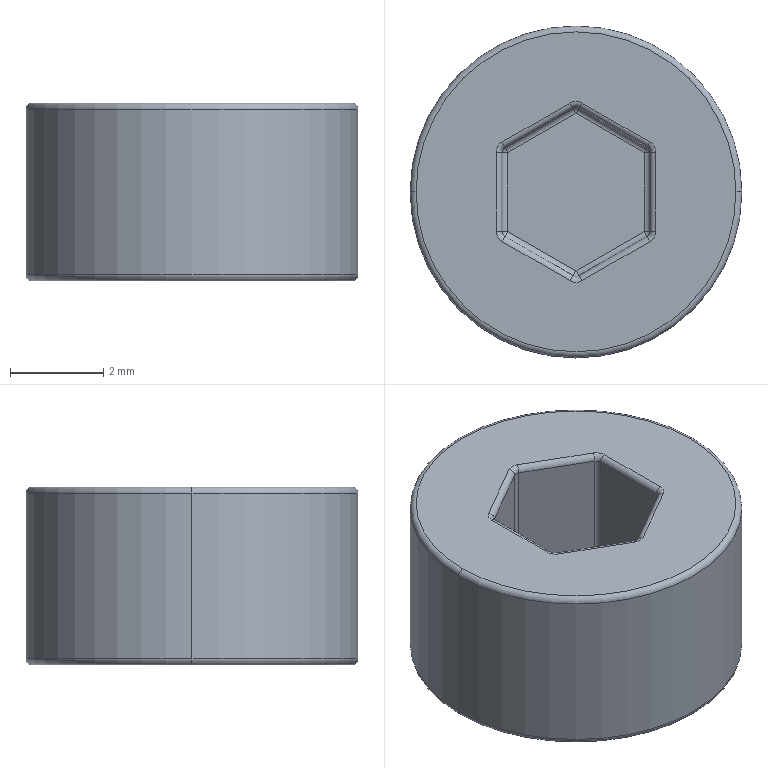Part | STEP file | BOLT | 1 solid | 45 faces | box 7.112 x 7.112 x 3.81 mm | volume 129.04 mm3 | cylinder 20 | torus 10 | plane 9 | sphere 6 | commonest cylinder face diameters 0.254 x18 7.112 x2
STEP:
#1=CARTESIAN_POINT('',(-3.556,0.,-0.127));
#2=VERTEX_POINT('',#1);
#3=CARTESIAN_POINT('',(3.556,0.,-0.127));
#4=VERTEX_POINT('',#3);
#5=CARTESIAN_POINT('',(0.,0.,-0.127));
#6=DIRECTION('',(0.,0.,-1.));
#7=DIRECTION('',(1.,0.,0.));
#8=AXIS2_PLACEMENT_3D('',#5,#6,#7);
#9=CIRCLE('',#8,3.556);
#10=EDGE_CURVE('',#2,#4,#9,.T.);
#11=ORIENTED_EDGE('',*,*,#10,.F.);
#12=CARTESIAN_POINT('',(-3.429,0.,0.));
#13=VERTEX_POINT('',#12);
#14=CARTESIAN_POINT('',(-3.429,0.,-0.127));
#15=DIRECTION('',(0.,1.,0.));
#16=DIRECTION('',(-1.,0.,0.));
#17=AXIS2_PLACEMENT_3D('',#14,#15,#16);
#18=CIRCLE('',#17,0.127);
#19=EDGE_CURVE('',#2,#13,#18,.T.);
#20=ORIENTED_EDGE('',*,*,#19,.T.);
#21=CARTESIAN_POINT('',(3.429,0.,0.));
#22=VERTEX_POINT('',#21);
#23=CARTESIAN_POINT('',(0.,0.,0.));
#24=DIRECTION('',(0.,0.,1.));
#25=DIRECTION('',(1.,0.,0.));
#26=AXIS2_PLACEMENT_3D('',#23,#24,#25);
#27=CIRCLE('',#26,3.429);
#28=EDGE_CURVE('',#22,#13,#27,.T.);
#29=ORIENTED_EDGE('',*,*,#28,.F.);
#30=CARTESIAN_POINT('',(3.429,0.,-0.127));
#31=DIRECTION('',(0.,-1.,0.));
#32=DIRECTION('',(0.,0.,-1.));
#33=AXIS2_PLACEMENT_3D('',#30,#31,#32);
#34=CIRCLE('',#33,0.127);
#35=EDGE_CURVE('',#4,#22,#34,.T.);
#36=ORIENTED_EDGE('',*,*,#35,.F.);
#37=EDGE_LOOP('',(#11,#20,#29,#36));
#38=FACE_OUTER_BOUND('',#37,.T.);
#39=CARTESIAN_POINT('',(0.,0.,-0.127));
#40=DIRECTION('',(0.,0.,1.));
#41=DIRECTION('',(1.,0.,0.));
#42=AXIS2_PLACEMENT_3D('',#39,#40,#41);
#43=TOROIDAL_SURFACE('',#42,3.429,0.127);
#44=ADVANCED_FACE('',(#38),#43,.T.);
#45=CARTESIAN_POINT('',(-3.429,0.,-3.81));
#46=VERTEX_POINT('',#45);
#47=CARTESIAN_POINT('',(3.429,0.,-3.81));
#48=VERTEX_POINT('',#47);
#49=CARTESIAN_POINT('',(0.,0.,-3.81));
#50=DIRECTION('',(0.,0.,-1.));
#51=DIRECTION('',(1.,0.,0.));
#52=AXIS2_PLACEMENT_3D('',#49,#50,#51);
#53=CIRCLE('',#52,3.429);
#54=EDGE_CURVE('',#46,#48,#53,.T.);
#55=ORIENTED_EDGE('',*,*,#54,.F.);
#56=CARTESIAN_POINT('',(-3.556,0.,-3.683));
#57=VERTEX_POINT('',#56);
#58=CARTESIAN_POINT('',(-3.429,0.,-3.683));
#59=DIRECTION('',(0.,1.,0.));
#60=DIRECTION('',(-1.,0.,0.));
#61=AXIS2_PLACEMENT_3D('',#58,#59,#60);
#62=CIRCLE('',#61,0.127);
#63=EDGE_CURVE('',#46,#57,#62,.T.);
#64=ORIENTED_EDGE('',*,*,#63,.T.);
#65=CARTESIAN_POINT('',(3.556,0.,-3.683));
#66=VERTEX_POINT('',#65);
#67=CARTESIAN_POINT('',(0.,0.,-3.683));
#68=DIRECTION('',(0.,0.,1.));
#69=DIRECTION('',(1.,0.,0.));
#70=AXIS2_PLACEMENT_3D('',#67,#68,#69);
#71=CIRCLE('',#70,3.556);
#72=EDGE_CURVE('',#66,#57,#71,.T.);
#73=ORIENTED_EDGE('',*,*,#72,.F.);
#74=CARTESIAN_POINT('',(3.429,0.,-3.683));
#75=DIRECTION('',(0.,-1.,0.));
#76=DIRECTION('',(0.,0.,-1.));
#77=AXIS2_PLACEMENT_3D('',#74,#75,#76);
#78=CIRCLE('',#77,0.127);
#79=EDGE_CURVE('',#48,#66,#78,.T.);
#80=ORIENTED_EDGE('',*,*,#79,.F.);
#81=EDGE_LOOP('',(#55,#64,#73,#80));
#82=FACE_OUTER_BOUND('',#81,.T.);
#83=CARTESIAN_POINT('',(0.,0.,-3.683));
#84=DIRECTION('',(0.,0.,1.));
#85=DIRECTION('',(1.,0.,0.));
#86=AXIS2_PLACEMENT_3D('',#83,#84,#85);
#87=TOROIDAL_SURFACE('',#86,3.429,0.127);
#88=ADVANCED_FACE('',(#82),#87,.T.);
#89=ORIENTED_EDGE('',*,*,#72,.T.);
#90=CARTESIAN_POINT('',(-3.556,0.,-3.81));
#91=DIRECTION('',(0.,0.,1.));
#92=VECTOR('',#91,1000.);
#93=LINE('',#90,#92);
#94=EDGE_CURVE('',#57,#2,#93,.T.);
#95=ORIENTED_EDGE('',*,*,#94,.T.);
#96=ORIENTED_EDGE('',*,*,#10,.T.);
#97=CARTESIAN_POINT('',(3.556,0.,-3.81));
#98=DIRECTION('',(0.,0.,1.));
#99=VECTOR('',#98,1000.);
#100=LINE('',#97,#99);
#101=EDGE_CURVE('',#66,#4,#100,.T.);
#102=ORIENTED_EDGE('',*,*,#101,.F.);
#103=EDGE_LOOP('',(#89,#95,#96,#102));
#104=FACE_OUTER_BOUND('',#103,.T.);
#105=CARTESIAN_POINT('',(0.,0.,-3.81));
#106=DIRECTION('',(0.,0.,1.));
#107=DIRECTION('',(1.,0.,0.));
#108=AXIS2_PLACEMENT_3D('',#105,#106,#107);
#109=CYLINDRICAL_SURFACE('',#108,3.556);
#110=ADVANCED_FACE('',(#104),#109,.T.);
#111=ORIENTED_EDGE('',*,*,#28,.T.);
#112=CARTESIAN_POINT('',(0.,0.,0.));
#113=DIRECTION('',(0.,0.,1.));
#114=DIRECTION('',(1.,0.,0.));
#115=AXIS2_PLACEMENT_3D('',#112,#113,#114);
#116=CIRCLE('',#115,3.429);
#117=EDGE_CURVE('',#13,#22,#116,.T.);
#118=ORIENTED_EDGE('',*,*,#117,.T.);
#119=EDGE_LOOP('',(#111,#118));
#120=FACE_OUTER_BOUND('',#119,.T.);
#121=CARTESIAN_POINT('',(1.587,-1.063,0.));
#122=VERTEX_POINT('',#121);
#123=CARTESIAN_POINT('',(1.715,-0.8432,0.));
#124=VERTEX_POINT('',#123);
#125=CARTESIAN_POINT('',(1.46,-0.8432,0.));
#126=DIRECTION('',(0.,0.,1.));
#127=DIRECTION('',(1.,0.,0.));
#128=AXIS2_PLACEMENT_3D('',#125,#126,#127);
#129=CIRCLE('',#128,0.254);
#130=EDGE_CURVE('',#122,#124,#129,.T.);
#131=ORIENTED_EDGE('',*,*,#130,.F.);
#132=CARTESIAN_POINT('',(0.127,-1.906,0.));
#133=VERTEX_POINT('',#132);
#134=CARTESIAN_POINT('',(0.8573,-1.485,0.));
#135=DIRECTION('',(-0.866,-0.5,0.));
#136=VECTOR('',#135,1000.);
#137=LINE('',#134,#136);
#138=EDGE_CURVE('',#122,#133,#137,.T.);
#139=ORIENTED_EDGE('',*,*,#138,.T.);
#140=CARTESIAN_POINT('',(-0.127,-1.906,0.));
#141=VERTEX_POINT('',#140);
#142=CARTESIAN_POINT('',(0.,-1.686,0.));
#143=DIRECTION('',(0.,0.,1.));
#144=DIRECTION('',(1.,0.,0.));
#145=AXIS2_PLACEMENT_3D('',#142,#143,#144);
#146=CIRCLE('',#145,0.254);
#147=EDGE_CURVE('',#141,#133,#146,.T.);
#148=ORIENTED_EDGE('',*,*,#147,.F.);
#149=CARTESIAN_POINT('',(-1.587,-1.063,0.));
#150=VERTEX_POINT('',#149);
#151=CARTESIAN_POINT('',(-0.8573,-1.485,0.));
#152=DIRECTION('',(-0.866,0.5,0.));
#153=VECTOR('',#152,1000.);
#154=LINE('',#151,#153);
#155=EDGE_CURVE('',#141,#150,#154,.T.);
#156=ORIENTED_EDGE('',*,*,#155,.T.);
#157=CARTESIAN_POINT('',(-1.715,-0.8432,0.));
#158=VERTEX_POINT('',#157);
#159=CARTESIAN_POINT('',(-1.46,-0.8432,0.));
#160=DIRECTION('',(0.,0.,1.));
#161=DIRECTION('',(1.,0.,0.));
#162=AXIS2_PLACEMENT_3D('',#159,#160,#161);
#163=CIRCLE('',#162,0.254);
#164=EDGE_CURVE('',#158,#150,#163,.T.);
#165=ORIENTED_EDGE('',*,*,#164,.F.);
#166=CARTESIAN_POINT('',(-1.715,0.8432,0.));
#167=VERTEX_POINT('',#166);
#168=CARTESIAN_POINT('',(-1.715,0.,0.));
#169=DIRECTION('',(0.,1.,0.));
#170=VECTOR('',#169,1000.);
#171=LINE('',#168,#170);
#172=EDGE_CURVE('',#158,#167,#171,.T.);
#173=ORIENTED_EDGE('',*,*,#172,.T.);
#174=CARTESIAN_POINT('',(-1.587,1.063,0.));
#175=VERTEX_POINT('',#174);
#176=CARTESIAN_POINT('',(-1.46,0.8432,0.));
#177=DIRECTION('',(0.,0.,1.));
#178=DIRECTION('',(1.,0.,0.));
#179=AXIS2_PLACEMENT_3D('',#176,#177,#178);
#180=CIRCLE('',#179,0.254);
#181=EDGE_CURVE('',#175,#167,#180,.T.);
#182=ORIENTED_EDGE('',*,*,#181,.F.);
#183=CARTESIAN_POINT('',(-0.127,1.906,0.));
#184=VERTEX_POINT('',#183);
#185=CARTESIAN_POINT('',(-0.8573,1.485,0.));
#186=DIRECTION('',(0.866,0.5,0.));
#187=VECTOR('',#186,1000.);
#188=LINE('',#185,#187);
#189=EDGE_CURVE('',#175,#184,#188,.T.);
#190=ORIENTED_EDGE('',*,*,#189,.T.);
#191=CARTESIAN_POINT('',(0.127,1.906,0.));
#192=VERTEX_POINT('',#191);
#193=CARTESIAN_POINT('',(0.,1.686,0.));
#194=DIRECTION('',(0.,0.,1.));
#195=DIRECTION('',(1.,0.,0.));
#196=AXIS2_PLACEMENT_3D('',#193,#194,#195);
#197=CIRCLE('',#196,0.254);
#198=EDGE_CURVE('',#192,#184,#197,.T.);
#199=ORIENTED_EDGE('',*,*,#198,.F.);
#200=CARTESIAN_POINT('',(1.587,1.063,0.));
#201=VERTEX_POINT('',#200);
#202=CARTESIAN_POINT('',(0.8573,1.485,0.));
#203=DIRECTION('',(0.866,-0.5,0.));
#204=VECTOR('',#203,1000.);
#205=LINE('',#202,#204);
#206=EDGE_CURVE('',#192,#201,#205,.T.);
#207=ORIENTED_EDGE('',*,*,#206,.T.);
#208=CARTESIAN_POINT('',(1.715,0.8432,0.));
#209=VERTEX_POINT('',#208);
#210=CARTESIAN_POINT('',(1.46,0.8432,0.));
#211=DIRECTION('',(0.,0.,1.));
#212=DIRECTION('',(1.,0.,0.));
#213=AXIS2_PLACEMENT_3D('',#210,#211,#212);
#214=CIRCLE('',#213,0.254);
#215=EDGE_CURVE('',#209,#201,#214,.T.);
#216=ORIENTED_EDGE('',*,*,#215,.F.);
#217=CARTESIAN_POINT('',(1.715,0.,0.));
#218=DIRECTION('',(0.,-1.,0.));
#219=VECTOR('',#218,1000.);
#220=LINE('',#217,#219);
#221=EDGE_CURVE('',#209,#124,#220,.T.);
#222=ORIENTED_EDGE('',*,*,#221,.T.);
#223=EDGE_LOOP('',(#131,#139,#148,#156,#165,#173,#182,#190,#199,#207,#216,#222));
#224=FACE_BOUND('',#223,.T.);
#225=CARTESIAN_POINT('',(0.,0.,0.));
#226=DIRECTION('',(0.,0.,1.));
#227=DIRECTION('',(1.,0.,0.));
#228=AXIS2_PLACEMENT_3D('',#225,#226,#227);
#229=PLANE('',#228);
#230=ADVANCED_FACE('',(#120,#224),#229,.T.);
#231=ORIENTED_EDGE('',*,*,#94,.F.);
#232=CARTESIAN_POINT('',(0.,0.,-3.683));
#233=DIRECTION('',(0.,0.,1.));
#234=DIRECTION('',(1.,0.,0.));
#235=AXIS2_PLACEMENT_3D('',#232,#233,#234);
#236=CIRCLE('',#235,3.556);
#237=EDGE_CURVE('',#57,#66,#236,.T.);
#238=ORIENTED_EDGE('',*,*,#237,.T.);
#239=ORIENTED_EDGE('',*,*,#101,.T.);
#240=CARTESIAN_POINT('',(0.,0.,-0.127));
#241=DIRECTION('',(0.,0.,-1.));
#242=DIRECTION('',(1.,0.,0.));
#243=AXIS2_PLACEMENT_3D('',#240,#241,#242);
#244=CIRCLE('',#243,3.556);
#245=EDGE_CURVE('',#4,#2,#244,.T.);
#246=ORIENTED_EDGE('',*,*,#245,.T.);
#247=EDGE_LOOP('',(#231,#238,#239,#246));
#248=FACE_OUTER_BOUND('',#247,.T.);
#249=CARTESIAN_POINT('',(0.,0.,-3.81));
#250=DIRECTION('',(0.,0.,1.));
#251=DIRECTION('',(1.,0.,0.));
#252=AXIS2_PLACEMENT_3D('',#249,#250,#251);
#253=CYLINDRICAL_SURFACE('',#252,3.556);
#254=ADVANCED_FACE('',(#248),#253,.T.);
#255=CARTESIAN_POINT('',(0.,0.,-3.81));
#256=DIRECTION('',(0.,0.,-1.));
#257=DIRECTION('',(1.,0.,0.));
#258=AXIS2_PLACEMENT_3D('',#255,#256,#257);
#259=CIRCLE('',#258,3.429);
#260=EDGE_CURVE('',#48,#46,#259,.T.);
#261=ORIENTED_EDGE('',*,*,#260,.T.);
#262=ORIENTED_EDGE('',*,*,#54,.T.);
#263=EDGE_LOOP('',(#261,#262));
#264=FACE_OUTER_BOUND('',#263,.T.);
#265=CARTESIAN_POINT('',(0.,0.,-3.81));
#266=DIRECTION('',(0.,0.,1.));
#267=DIRECTION('',(1.,0.,0.));
#268=AXIS2_PLACEMENT_3D('',#265,#266,#267);
#269=PLANE('',#268);
#270=ADVANCED_FACE('',(#264),#269,.F.);
#271=CARTESIAN_POINT('',(-1.587,0.8432,-0.127));
#272=VERTEX_POINT('',#271);
#273=CARTESIAN_POINT('',(-1.587,-0.8432,-0.127));
#274=VERTEX_POINT('',#273);
#275=CARTESIAN_POINT('',(-1.587,0.9165,-0.127));
#276=DIRECTION('',(0.,-1.,0.));
#277=VECTOR('',#276,1000.);
#278=LINE('',#275,#277);
#279=EDGE_CURVE('',#272,#274,#278,.T.);
#280=ORIENTED_EDGE('',*,*,#279,.T.);
#281=CARTESIAN_POINT('',(-1.587,-0.8432,-2.413));
#282=VERTEX_POINT('',#281);
#283=CARTESIAN_POINT('',(-1.587,-0.8432,-2.54));
#284=DIRECTION('',(0.,0.,-1.));
#285=VECTOR('',#284,1000.);
#286=LINE('',#283,#285);
#287=EDGE_CURVE('',#274,#282,#286,.T.);
#288=ORIENTED_EDGE('',*,*,#287,.T.);
#289=CARTESIAN_POINT('',(-1.587,0.8432,-2.413));
#290=VERTEX_POINT('',#289);
#291=CARTESIAN_POINT('',(-1.587,0.9165,-2.413));
#292=DIRECTION('',(0.,1.,0.));
#293=VECTOR('',#292,1000.);
#294=LINE('',#291,#293);
#295=EDGE_CURVE('',#282,#290,#294,.T.);
#296=ORIENTED_EDGE('',*,*,#295,.T.);
#297=CARTESIAN_POINT('',(-1.587,0.8432,0.));
#298=DIRECTION('',(0.,0.,1.));
#299=VECTOR('',#298,1000.);
#300=LINE('',#297,#299);
#301=EDGE_CURVE('',#290,#272,#300,.T.);
#302=ORIENTED_EDGE('',*,*,#301,.T.);
#303=EDGE_LOOP('',(#280,#288,#296,#302));
#304=FACE_OUTER_BOUND('',#303,.T.);
#305=CARTESIAN_POINT('',(-1.587,0.9165,2.54));
#306=DIRECTION('',(1.,0.,0.));
#307=DIRECTION('',(0.,1.,0.));
#308=AXIS2_PLACEMENT_3D('',#305,#306,#307);
#309=PLANE('',#308);
#310=ADVANCED_FACE('',(#304),#309,.T.);
#311=CARTESIAN_POINT('',(-1.524,-0.9532,-2.413));
#312=VERTEX_POINT('',#311);
#313=CARTESIAN_POINT('',(-1.524,-0.9532,-0.127));
#314=VERTEX_POINT('',#313);
#315=CARTESIAN_POINT('',(-1.524,-0.9532,0.));
#316=DIRECTION('',(0.,0.,1.));
#317=VECTOR('',#316,1000.);
#318=LINE('',#315,#317);
#319=EDGE_CURVE('',#312,#314,#318,.T.);
#320=ORIENTED_EDGE('',*,*,#319,.T.);
#321=CARTESIAN_POINT('',(-0.0635,-1.796,-0.127));
#322=VERTEX_POINT('',#321);
#323=CARTESIAN_POINT('',(-1.587,-0.9165,-0.127));
#324=DIRECTION('',(0.866,-0.5,0.));
#325=VECTOR('',#324,1000.);
#326=LINE('',#323,#325);
#327=EDGE_CURVE('',#314,#322,#326,.T.);
#328=ORIENTED_EDGE('',*,*,#327,.T.);
#329=CARTESIAN_POINT('',(-0.0635,-1.796,-2.413));
#330=VERTEX_POINT('',#329);
#331=CARTESIAN_POINT('',(-0.0635,-1.796,-2.54));
#332=DIRECTION('',(0.,0.,-1.));
#333=VECTOR('',#332,1000.);
#334=LINE('',#331,#333);
#335=EDGE_CURVE('',#322,#330,#334,.T.);
#336=ORIENTED_EDGE('',*,*,#335,.T.);
#337=CARTESIAN_POINT('',(-1.587,-0.9165,-2.413));
#338=DIRECTION('',(-0.866,0.5,0.));
#339=VECTOR('',#338,1000.);
#340=LINE('',#337,#339);
#341=EDGE_CURVE('',#330,#312,#340,.T.);
#342=ORIENTED_EDGE('',*,*,#341,.T.);
#343=EDGE_LOOP('',(#320,#328,#336,#342));
#344=FACE_OUTER_BOUND('',#343,.T.);
#345=CARTESIAN_POINT('',(-1.587,-0.9165,2.54));
#346=DIRECTION('',(0.5,0.866,0.));
#347=DIRECTION('',(-0.866,0.5,0.));
#348=AXIS2_PLACEMENT_3D('',#345,#346,#347);
#349=PLANE('',#348);
#350=ADVANCED_FACE('',(#344),#349,.T.);
#351=CARTESIAN_POINT('',(0.0635,-1.796,-2.413));
#352=VERTEX_POINT('',#351);
#353=CARTESIAN_POINT('',(0.0635,-1.796,-0.127));
#354=VERTEX_POINT('',#353);
#355=CARTESIAN_POINT('',(0.0635,-1.796,0.));
#356=DIRECTION('',(0.,0.,1.));
#357=VECTOR('',#356,1000.);
#358=LINE('',#355,#357);
#359=EDGE_CURVE('',#352,#354,#358,.T.);
#360=ORIENTED_EDGE('',*,*,#359,.T.);
#361=CARTESIAN_POINT('',(1.524,-0.9532,-0.127));
#362=VERTEX_POINT('',#361);
#363=CARTESIAN_POINT('',(0.,-1.833,-0.127));
#364=DIRECTION('',(0.866,0.5,0.));
#365=VECTOR('',#364,1000.);
#366=LINE('',#363,#365);
#367=EDGE_CURVE('',#354,#362,#366,.T.);
#368=ORIENTED_EDGE('',*,*,#367,.T.);
#369=CARTESIAN_POINT('',(1.524,-0.9532,-2.413));
#370=VERTEX_POINT('',#369);
#371=CARTESIAN_POINT('',(1.524,-0.9532,-2.54));
#372=DIRECTION('',(0.,0.,-1.));
#373=VECTOR('',#372,1000.);
#374=LINE('',#371,#373);
#375=EDGE_CURVE('',#362,#370,#374,.T.);
#376=ORIENTED_EDGE('',*,*,#375,.T.);
#377=CARTESIAN_POINT('',(0.,-1.833,-2.413));
#378=DIRECTION('',(-0.866,-0.5,0.));
#379=VECTOR('',#378,1000.);
#380=LINE('',#377,#379);
#381=EDGE_CURVE('',#370,#352,#380,.T.);
#382=ORIENTED_EDGE('',*,*,#381,.T.);
#383=EDGE_LOOP('',(#360,#368,#376,#382));
#384=FACE_OUTER_BOUND('',#383,.T.);
#385=CARTESIAN_POINT('',(0.,-1.833,2.54));
#386=DIRECTION('',(-0.5,0.866,0.));
#387=DIRECTION('',(-0.866,-0.5,0.));
#388=AXIS2_PLACEMENT_3D('',#385,#386,#387);
#389=PLANE('',#388);
#390=ADVANCED_FACE('',(#384),#389,.T.);
#391=CARTESIAN_POINT('',(1.587,-0.8432,-2.413));
#392=VERTEX_POINT('',#391);
#393=CARTESIAN_POINT('',(1.587,-0.8432,-0.127));
#394=VERTEX_POINT('',#393);
#395=CARTESIAN_POINT('',(1.587,-0.8432,0.));
#396=DIRECTION('',(0.,0.,1.));
#397=VECTOR('',#396,1000.);
#398=LINE('',#395,#397);
#399=EDGE_CURVE('',#392,#394,#398,.T.);
#400=ORIENTED_EDGE('',*,*,#399,.T.);
#401=CARTESIAN_POINT('',(1.587,0.8432,-0.127));
#402=VERTEX_POINT('',#401);
#403=CARTESIAN_POINT('',(1.587,-0.9165,-0.127));
#404=DIRECTION('',(0.,1.,0.));
#405=VECTOR('',#404,1000.);
#406=LINE('',#403,#405);
#407=EDGE_CURVE('',#394,#402,#406,.T.);
#408=ORIENTED_EDGE('',*,*,#407,.T.);
#409=CARTESIAN_POINT('',(1.587,0.8432,-2.413));
#410=VERTEX_POINT('',#409);
#411=CARTESIAN_POINT('',(1.587,0.8432,-2.54));
#412=DIRECTION('',(0.,0.,-1.));
#413=VECTOR('',#412,1000.);
#414=LINE('',#411,#413);
#415=EDGE_CURVE('',#402,#410,#414,.T.);
#416=ORIENTED_EDGE('',*,*,#415,.T.);
#417=CARTESIAN_POINT('',(1.587,-0.9165,-2.413));
#418=DIRECTION('',(0.,-1.,0.));
#419=VECTOR('',#418,1000.);
#420=LINE('',#417,#419);
#421=EDGE_CURVE('',#410,#392,#420,.T.);
#422=ORIENTED_EDGE('',*,*,#421,.T.);
#423=EDGE_LOOP('',(#400,#408,#416,#422));
#424=FACE_OUTER_BOUND('',#423,.T.);
#425=CARTESIAN_POINT('',(1.587,-0.9165,2.54));
#426=DIRECTION('',(-1.,0.,0.));
#427=DIRECTION('',(0.,-1.,0.));
#428=AXIS2_PLACEMENT_3D('',#425,#426,#427);
#429=PLANE('',#428);
#430=ADVANCED_FACE('',(#424),#429,.T.);
#431=CARTESIAN_POINT('',(1.524,0.9532,-2.413));
#432=VERTEX_POINT('',#431);
#433=CARTESIAN_POINT('',(1.524,0.9532,-0.127));
#434=VERTEX_POINT('',#433);
#435=CARTESIAN_POINT('',(1.524,0.9532,0.));
#436=DIRECTION('',(0.,0.,1.));
#437=VECTOR('',#436,1000.);
#438=LINE('',#435,#437);
#439=EDGE_CURVE('',#432,#434,#438,.T.);
#440=ORIENTED_EDGE('',*,*,#439,.T.);
#441=CARTESIAN_POINT('',(0.0635,1.796,-0.127));
#442=VERTEX_POINT('',#441);
#443=CARTESIAN_POINT('',(1.587,0.9165,-0.127));
#444=DIRECTION('',(-0.866,0.5,0.));
#445=VECTOR('',#444,1000.);
#446=LINE('',#443,#445);
#447=EDGE_CURVE('',#434,#442,#446,.T.);
#448=ORIENTED_EDGE('',*,*,#447,.T.);
#449=CARTESIAN_POINT('',(0.0635,1.796,-2.413));
#450=VERTEX_POINT('',#449);
#451=CARTESIAN_POINT('',(0.0635,1.796,-2.54));
#452=DIRECTION('',(0.,0.,-1.));
#453=VECTOR('',#452,1000.);
#454=LINE('',#451,#453);
#455=EDGE_CURVE('',#442,#450,#454,.T.);
#456=ORIENTED_EDGE('',*,*,#455,.T.);
#457=CARTESIAN_POINT('',(1.587,0.9165,-2.413));
#458=DIRECTION('',(0.866,-0.5,0.));
#459=VECTOR('',#458,1000.);
#460=LINE('',#457,#459);
#461=EDGE_CURVE('',#450,#432,#460,.T.);
#462=ORIENTED_EDGE('',*,*,#461,.T.);
#463=EDGE_LOOP('',(#440,#448,#456,#462));
#464=FACE_OUTER_BOUND('',#463,.T.);
#465=CARTESIAN_POINT('',(1.587,0.9165,2.54));
#466=DIRECTION('',(-0.5,-0.866,0.));
#467=DIRECTION('',(0.866,-0.5,0.));
#468=AXIS2_PLACEMENT_3D('',#465,#466,#467);
#469=PLANE('',#468);
#470=ADVANCED_FACE('',(#464),#469,.T.);
#471=CARTESIAN_POINT('',(-0.0635,1.796,-2.413));
#472=VERTEX_POINT('',#471);
#473=CARTESIAN_POINT('',(-0.0635,1.796,-0.127));
#474=VERTEX_POINT('',#473);
#475=CARTESIAN_POINT('',(-0.0635,1.796,0.));
#476=DIRECTION('',(0.,0.,1.));
#477=VECTOR('',#476,1000.);
#478=LINE('',#475,#477);
#479=EDGE_CURVE('',#472,#474,#478,.T.);
#480=ORIENTED_EDGE('',*,*,#479,.T.);
#481=CARTESIAN_POINT('',(-1.524,0.9532,-0.127));
#482=VERTEX_POINT('',#481);
#483=CARTESIAN_POINT('',(0.,1.833,-0.127));
#484=DIRECTION('',(-0.866,-0.5,0.));
#485=VECTOR('',#484,1000.);
#486=LINE('',#483,#485);
#487=EDGE_CURVE('',#474,#482,#486,.T.);
#488=ORIENTED_EDGE('',*,*,#487,.T.);
#489=CARTESIAN_POINT('',(-1.524,0.9532,-2.413));
#490=VERTEX_POINT('',#489);
#491=CARTESIAN_POINT('',(-1.524,0.9532,-2.54));
#492=DIRECTION('',(0.,0.,-1.));
#493=VECTOR('',#492,1000.);
#494=LINE('',#491,#493);
#495=EDGE_CURVE('',#482,#490,#494,.T.);
#496=ORIENTED_EDGE('',*,*,#495,.T.);
#497=CARTESIAN_POINT('',(0.,1.833,-2.413));
#498=DIRECTION('',(0.866,0.5,0.));
#499=VECTOR('',#498,1000.);
#500=LINE('',#497,#499);
#501=EDGE_CURVE('',#490,#472,#500,.T.);
#502=ORIENTED_EDGE('',*,*,#501,.T.);
#503=EDGE_LOOP('',(#480,#488,#496,#502));
#504=FACE_OUTER_BOUND('',#503,.T.);
#505=CARTESIAN_POINT('',(0.,1.833,2.54));
#506=DIRECTION('',(0.5,-0.866,0.));
#507=DIRECTION('',(0.866,0.5,0.));
#508=AXIS2_PLACEMENT_3D('',#505,#506,#507);
#509=PLANE('',#508);
#510=ADVANCED_FACE('',(#504),#509,.T.);
#511=CARTESIAN_POINT('',(0.,1.686,-2.54));
#512=VERTEX_POINT('',#511);
#513=CARTESIAN_POINT('',(-1.46,0.8432,-2.54));
#514=VERTEX_POINT('',#513);
#515=CARTESIAN_POINT('',(-1.524,0.8066,-2.54));
#516=DIRECTION('',(-0.866,-0.5,0.));
#517=VECTOR('',#516,1000.);
#518=LINE('',#515,#517);
#519=EDGE_CURVE('',#512,#514,#518,.T.);
#520=ORIENTED_EDGE('',*,*,#519,.T.);
#521=CARTESIAN_POINT('',(-1.46,-0.8432,-2.54));
#522=VERTEX_POINT('',#521);
#523=CARTESIAN_POINT('',(-1.46,-0.9165,-2.54));
#524=DIRECTION('',(0.,-1.,0.));
#525=VECTOR('',#524,1000.);
#526=LINE('',#523,#525);
#527=EDGE_CURVE('',#514,#522,#526,.T.);
#528=ORIENTED_EDGE('',*,*,#527,.T.);
#529=CARTESIAN_POINT('',(0.,-1.686,-2.54));
#530=VERTEX_POINT('',#529);
#531=CARTESIAN_POINT('',(0.0635,-1.723,-2.54));
#532=DIRECTION('',(0.866,-0.5,0.));
#533=VECTOR('',#532,1000.);
#534=LINE('',#531,#533);
#535=EDGE_CURVE('',#522,#530,#534,.T.);
#536=ORIENTED_EDGE('',*,*,#535,.T.);
#537=CARTESIAN_POINT('',(1.46,-0.8432,-2.54));
#538=VERTEX_POINT('',#537);
#539=CARTESIAN_POINT('',(1.524,-0.8066,-2.54));
#540=DIRECTION('',(0.866,0.5,0.));
#541=VECTOR('',#540,1000.);
#542=LINE('',#539,#541);
#543=EDGE_CURVE('',#530,#538,#542,.T.);
#544=ORIENTED_EDGE('',*,*,#543,.T.);
#545=CARTESIAN_POINT('',(1.46,0.8432,-2.54));
#546=VERTEX_POINT('',#545);
#547=CARTESIAN_POINT('',(1.46,0.9165,-2.54));
#548=DIRECTION('',(0.,1.,0.));
#549=VECTOR('',#548,1000.);
#550=LINE('',#547,#549);
#551=EDGE_CURVE('',#538,#546,#550,.T.);
#552=ORIENTED_EDGE('',*,*,#551,.T.);
#553=CARTESIAN_POINT('',(-0.0635,1.723,-2.54));
#554=DIRECTION('',(-0.866,0.5,0.));
#555=VECTOR('',#554,1000.);
#556=LINE('',#553,#555);
#557=EDGE_CURVE('',#546,#512,#556,.T.);
#558=ORIENTED_EDGE('',*,*,#557,.T.);
#559=EDGE_LOOP('',(#520,#528,#536,#544,#552,#558));
#560=FACE_OUTER_BOUND('',#559,.T.);
#561=CARTESIAN_POINT('',(-1.587,-0.9165,-2.54));
#562=DIRECTION('',(0.,0.,1.));
#563=DIRECTION('',(1.,0.,0.));
#564=AXIS2_PLACEMENT_3D('',#561,#562,#563);
#565=PLANE('',#564);
#566=ADVANCED_FACE('',(#560),#565,.T.);
#567=ORIENTED_EDGE('',*,*,#63,.F.);
#568=ORIENTED_EDGE('',*,*,#260,.F.);
#569=ORIENTED_EDGE('',*,*,#79,.T.);
#570=ORIENTED_EDGE('',*,*,#237,.F.);
#571=EDGE_LOOP('',(#567,#568,#569,#570));
#572=FACE_OUTER_BOUND('',#571,.T.);
#573=CARTESIAN_POINT('',(0.,0.,-3.683));
#574=DIRECTION('',(0.,0.,1.));
#575=DIRECTION('',(1.,0.,0.));
#576=AXIS2_PLACEMENT_3D('',#573,#574,#575);
#577=TOROIDAL_SURFACE('',#576,3.429,0.127);
#578=ADVANCED_FACE('',(#572),#577,.T.);
#579=CARTESIAN_POINT('',(1.46,-0.8432,-2.413));
#580=DIRECTION('',(0.,1.,0.));
#581=DIRECTION('',(-1.,0.,0.));
#582=AXIS2_PLACEMENT_3D('',#579,#580,#581);
#583=CIRCLE('',#582,0.127);
#584=EDGE_CURVE('',#392,#538,#583,.T.);
#585=ORIENTED_EDGE('',*,*,#584,.F.);
#586=ORIENTED_EDGE('',*,*,#421,.F.);
#587=CARTESIAN_POINT('',(1.46,0.8432,-2.413));
#588=DIRECTION('',(0.,-1.,0.));
#589=DIRECTION('',(1.,0.,0.));
#590=AXIS2_PLACEMENT_3D('',#587,#588,#589);
#591=CIRCLE('',#590,0.127);
#592=EDGE_CURVE('',#546,#410,#591,.T.);
#593=ORIENTED_EDGE('',*,*,#592,.F.);
#594=ORIENTED_EDGE('',*,*,#551,.F.);
#595=EDGE_LOOP('',(#585,#586,#593,#594));
#596=FACE_OUTER_BOUND('',#595,.T.);
#597=CARTESIAN_POINT('',(1.46,-0.9165,-2.413));
#598=DIRECTION('',(0.,-1.,0.));
#599=DIRECTION('',(1.,0.,0.));
#600=AXIS2_PLACEMENT_3D('',#597,#598,#599);
#601=CYLINDRICAL_SURFACE('',#600,0.127);
#602=ADVANCED_FACE('',(#596),#601,.F.);
#603=CARTESIAN_POINT('',(1.46,-0.8432,-2.413));
#604=DIRECTION('',(0.,0.,-1.));
#605=DIRECTION('',(1.,0.,0.));
#606=AXIS2_PLACEMENT_3D('',#603,#604,#605);
#607=CIRCLE('',#606,0.127);
#608=EDGE_CURVE('',#392,#370,#607,.T.);
#609=ORIENTED_EDGE('',*,*,#608,.F.);
#610=ORIENTED_EDGE('',*,*,#584,.T.);
#611=CARTESIAN_POINT('',(1.46,-0.8432,-2.413));
#612=DIRECTION('',(0.866,0.5,0.));
#613=DIRECTION('',(0.5,-0.866,0.));
#614=AXIS2_PLACEMENT_3D('',#611,#612,#613);
#615=CIRCLE('',#614,0.127);
#616=EDGE_CURVE('',#370,#538,#615,.T.);
#617=ORIENTED_EDGE('',*,*,#616,.F.);
#618=EDGE_LOOP('',(#609,#610,#617));
#619=FACE_OUTER_BOUND('',#618,.T.);
#620=CARTESIAN_POINT('',(1.46,-0.8432,-2.413));
#621=DIRECTION('',(0.,1.,0.));
#622=DIRECTION('',(1.,0.,0.));
#623=AXIS2_PLACEMENT_3D('',#620,#621,#622);
#624=SPHERICAL_SURFACE('',#623,0.127);
#625=ADVANCED_FACE('',(#619),#624,.F.);
#626=CARTESIAN_POINT('',(1.46,0.8432,-2.413));
#627=DIRECTION('',(0.866,-0.5,0.));
#628=DIRECTION('',(-0.5,-0.866,0.));
#629=AXIS2_PLACEMENT_3D('',#626,#627,#628);
#630=CIRCLE('',#629,0.127);
#631=EDGE_CURVE('',#546,#432,#630,.T.);
#632=ORIENTED_EDGE('',*,*,#631,.F.);
#633=ORIENTED_EDGE('',*,*,#592,.T.);
#634=CARTESIAN_POINT('',(1.46,0.8432,-2.413));
#635=DIRECTION('',(0.,0.,-1.));
#636=DIRECTION('',(1.,0.,0.));
#637=AXIS2_PLACEMENT_3D('',#634,#635,#636);
#638=CIRCLE('',#637,0.127);
#639=EDGE_CURVE('',#432,#410,#638,.T.);
#640=ORIENTED_EDGE('',*,*,#639,.F.);
#641=EDGE_LOOP('',(#632,#633,#640));
#642=FACE_OUTER_BOUND('',#641,.T.);
#643=CARTESIAN_POINT('',(1.46,0.8432,-2.413));
#644=DIRECTION('',(0.,1.,0.));
#645=DIRECTION('',(1.,0.,0.));
#646=AXIS2_PLACEMENT_3D('',#643,#644,#645);
#647=SPHERICAL_SURFACE('',#646,0.127);
#648=ADVANCED_FACE('',(#642),#647,.F.);
#649=ORIENTED_EDGE('',*,*,#616,.T.);
#650=ORIENTED_EDGE('',*,*,#543,.F.);
#651=CARTESIAN_POINT('',(0.,-1.686,-2.413));
#652=DIRECTION('',(0.866,0.5,0.));
#653=DIRECTION('',(-0.5,0.866,0.));
#654=AXIS2_PLACEMENT_3D('',#651,#652,#653);
#655=CIRCLE('',#654,0.127);
#656=EDGE_CURVE('',#352,#530,#655,.T.);
#657=ORIENTED_EDGE('',*,*,#656,.F.);
#658=ORIENTED_EDGE('',*,*,#381,.F.);
#659=EDGE_LOOP('',(#649,#650,#657,#658));
#660=FACE_OUTER_BOUND('',#659,.T.);
#661=CARTESIAN_POINT('',(-0.8573,-2.181,-2.413));
#662=DIRECTION('',(-0.866,-0.5,0.));
#663=DIRECTION('',(0.5,-0.866,0.));
#664=AXIS2_PLACEMENT_3D('',#661,#662,#663);
#665=CYLINDRICAL_SURFACE('',#664,0.127);
#666=ADVANCED_FACE('',(#660),#665,.F.);
#667=ORIENTED_EDGE('',*,*,#608,.T.);
#668=ORIENTED_EDGE('',*,*,#375,.F.);
#669=CARTESIAN_POINT('',(1.46,-0.8432,-0.127));
#670=DIRECTION('',(0.,0.,-1.));
#671=DIRECTION('',(1.,0.,0.));
#672=AXIS2_PLACEMENT_3D('',#669,#670,#671);
#673=CIRCLE('',#672,0.127);
#674=EDGE_CURVE('',#394,#362,#673,.T.);
#675=ORIENTED_EDGE('',*,*,#674,.F.);
#676=ORIENTED_EDGE('',*,*,#399,.F.);
#677=EDGE_LOOP('',(#667,#668,#675,#676));
#678=FACE_OUTER_BOUND('',#677,.T.);
#679=CARTESIAN_POINT('',(1.46,-0.8432,2.54));
#680=DIRECTION('',(0.,0.,1.));
#681=DIRECTION('',(1.,0.,0.));
#682=AXIS2_PLACEMENT_3D('',#679,#680,#681);
#683=CYLINDRICAL_SURFACE('',#682,0.127);
#684=ADVANCED_FACE('',(#678),#683,.F.);
#685=CARTESIAN_POINT('',(1.715,0.8432,-0.127));
#686=DIRECTION('',(0.,1.,0.));
#687=DIRECTION('',(-1.,0.,0.));
#688=AXIS2_PLACEMENT_3D('',#685,#686,#687);
#689=CIRCLE('',#688,0.127);
#690=EDGE_CURVE('',#402,#209,#689,.T.);
#691=ORIENTED_EDGE('',*,*,#690,.F.);
#692=ORIENTED_EDGE('',*,*,#407,.F.);
#693=CARTESIAN_POINT('',(1.715,-0.8432,-0.127));
#694=DIRECTION('',(0.,-1.,0.));
#695=DIRECTION('',(1.,0.,0.));
#696=AXIS2_PLACEMENT_3D('',#693,#694,#695);
#697=CIRCLE('',#696,0.127);
#698=EDGE_CURVE('',#124,#394,#697,.T.);
#699=ORIENTED_EDGE('',*,*,#698,.F.);
#700=ORIENTED_EDGE('',*,*,#221,.F.);
#701=EDGE_LOOP('',(#691,#692,#699,#700));
#702=FACE_OUTER_BOUND('',#701,.T.);
#703=CARTESIAN_POINT('',(1.715,0.,-0.127));
#704=DIRECTION('',(0.,-1.,0.));
#705=DIRECTION('',(1.,0.,0.));
#706=AXIS2_PLACEMENT_3D('',#703,#704,#705);
#707=CYLINDRICAL_SURFACE('',#706,0.127);
#708=ADVANCED_FACE('',(#702),#707,.T.);
#709=ORIENTED_EDGE('',*,*,#639,.T.);
#710=ORIENTED_EDGE('',*,*,#415,.F.);
#711=CARTESIAN_POINT('',(1.46,0.8432,-0.127));
#712=DIRECTION('',(0.,0.,-1.));
#713=DIRECTION('',(1.,0.,0.));
#714=AXIS2_PLACEMENT_3D('',#711,#712,#713);
#715=CIRCLE('',#714,0.127);
#716=EDGE_CURVE('',#434,#402,#715,.T.);
#717=ORIENTED_EDGE('',*,*,#716,.F.);
#718=ORIENTED_EDGE('',*,*,#439,.F.);
#719=EDGE_LOOP('',(#709,#710,#717,#718));
#720=FACE_OUTER_BOUND('',#719,.T.);
#721=CARTESIAN_POINT('',(1.46,0.8432,2.54));
#722=DIRECTION('',(0.,0.,1.));
#723=DIRECTION('',(1.,0.,0.));
#724=AXIS2_PLACEMENT_3D('',#721,#722,#723);
#725=CYLINDRICAL_SURFACE('',#724,0.127);
#726=ADVANCED_FACE('',(#720),#725,.F.);
#727=ORIENTED_EDGE('',*,*,#631,.T.);
#728=ORIENTED_EDGE('',*,*,#461,.F.);
#729=CARTESIAN_POINT('',(0.,1.686,-2.413));
#730=DIRECTION('',(0.866,-0.5,0.));
#731=DIRECTION('',(0.5,0.866,0.));
#732=AXIS2_PLACEMENT_3D('',#729,#730,#731);
#733=CIRCLE('',#732,0.127);
#734=EDGE_CURVE('',#512,#450,#733,.T.);
#735=ORIENTED_EDGE('',*,*,#734,.F.);
#736=ORIENTED_EDGE('',*,*,#557,.F.);
#737=EDGE_LOOP('',(#727,#728,#735,#736));
#738=FACE_OUTER_BOUND('',#737,.T.);
#739=CARTESIAN_POINT('',(-0.0635,1.723,-2.413));
#740=DIRECTION('',(0.866,-0.5,0.));
#741=DIRECTION('',(0.5,0.866,0.));
#742=AXIS2_PLACEMENT_3D('',#739,#740,#741);
#743=CYLINDRICAL_SURFACE('',#742,0.127);
#744=ADVANCED_FACE('',(#738),#743,.F.);
#745=CARTESIAN_POINT('',(0.,-1.686,-2.413));
#746=DIRECTION('',(0.,0.,-1.));
#747=DIRECTION('',(1.,0.,0.));
#748=AXIS2_PLACEMENT_3D('',#745,#746,#747);
#749=CIRCLE('',#748,0.127);
#750=EDGE_CURVE('',#352,#330,#749,.T.);
#751=ORIENTED_EDGE('',*,*,#750,.F.);
#752=ORIENTED_EDGE('',*,*,#656,.T.);
#753=CARTESIAN_POINT('',(0.,-1.686,-2.413));
#754=DIRECTION('',(0.866,-0.5,0.));
#755=DIRECTION('',(-0.5,-0.866,0.));
#756=AXIS2_PLACEMENT_3D('',#753,#754,#755);
#757=CIRCLE('',#756,0.127);
#758=EDGE_CURVE('',#330,#530,#757,.T.);
#759=ORIENTED_EDGE('',*,*,#758,.F.);
#760=EDGE_LOOP('',(#751,#752,#759));
#761=FACE_OUTER_BOUND('',#760,.T.);
#762=CARTESIAN_POINT('',(0.,-1.686,-2.413));
#763=DIRECTION('',(0.,1.,0.));
#764=DIRECTION('',(1.,0.,0.));
#765=AXIS2_PLACEMENT_3D('',#762,#763,#764);
#766=SPHERICAL_SURFACE('',#765,0.127);
#767=ADVANCED_FACE('',(#761),#766,.F.);
#768=ORIENTED_EDGE('',*,*,#698,.T.);
#769=ORIENTED_EDGE('',*,*,#674,.T.);
#770=CARTESIAN_POINT('',(1.587,-1.063,-0.127));
#771=DIRECTION('',(-0.866,-0.5,0.));
#772=DIRECTION('',(-0.5,0.866,0.));
#773=AXIS2_PLACEMENT_3D('',#770,#771,#772);
#774=CIRCLE('',#773,0.127);
#775=EDGE_CURVE('',#122,#362,#774,.T.);
#776=ORIENTED_EDGE('',*,*,#775,.F.);
#777=ORIENTED_EDGE('',*,*,#130,.T.);
#778=EDGE_LOOP('',(#768,#769,#776,#777));
#779=FACE_OUTER_BOUND('',#778,.T.);
#780=CARTESIAN_POINT('',(1.46,-0.8432,-0.127));
#781=DIRECTION('',(0.,0.,1.));
#782=DIRECTION('',(1.,0.,0.));
#783=AXIS2_PLACEMENT_3D('',#780,#781,#782);
#784=TOROIDAL_SURFACE('',#783,0.254,0.127);
#785=ADVANCED_FACE('',(#779),#784,.T.);
#786=ORIENTED_EDGE('',*,*,#690,.T.);
#787=ORIENTED_EDGE('',*,*,#215,.T.);
#788=CARTESIAN_POINT('',(1.587,1.063,-0.127));
#789=DIRECTION('',(-0.866,0.5,0.));
#790=DIRECTION('',(0.5,0.866,0.));
#791=AXIS2_PLACEMENT_3D('',#788,#789,#790);
#792=CIRCLE('',#791,0.127);
#793=EDGE_CURVE('',#434,#201,#792,.T.);
#794=ORIENTED_EDGE('',*,*,#793,.F.);
#795=ORIENTED_EDGE('',*,*,#716,.T.);
#796=EDGE_LOOP('',(#786,#787,#794,#795));
#797=FACE_OUTER_BOUND('',#796,.T.);
#798=CARTESIAN_POINT('',(1.46,0.8432,-0.127));
#799=DIRECTION('',(0.,0.,1.));
#800=DIRECTION('',(1.,0.,0.));
#801=AXIS2_PLACEMENT_3D('',#798,#799,#800);
#802=TOROIDAL_SURFACE('',#801,0.254,0.127);
#803=ADVANCED_FACE('',(#797),#802,.T.);
#804=CARTESIAN_POINT('',(0.,1.686,-2.413));
#805=DIRECTION('',(0.866,0.5,0.));
#806=DIRECTION('',(0.5,-0.866,0.));
#807=AXIS2_PLACEMENT_3D('',#804,#805,#806);
#808=CIRCLE('',#807,0.127);
#809=EDGE_CURVE('',#512,#472,#808,.T.);
#810=ORIENTED_EDGE('',*,*,#809,.F.);
#811=ORIENTED_EDGE('',*,*,#734,.T.);
#812=CARTESIAN_POINT('',(0.,1.686,-2.413));
#813=DIRECTION('',(0.,0.,-1.));
#814=DIRECTION('',(1.,0.,0.));
#815=AXIS2_PLACEMENT_3D('',#812,#813,#814);
#816=CIRCLE('',#815,0.127);
#817=EDGE_CURVE('',#472,#450,#816,.T.);
#818=ORIENTED_EDGE('',*,*,#817,.F.);
#819=EDGE_LOOP('',(#810,#811,#818));
#820=FACE_OUTER_BOUND('',#819,.T.);
#821=CARTESIAN_POINT('',(0.,1.686,-2.413));
#822=DIRECTION('',(0.,1.,0.));
#823=DIRECTION('',(1.,0.,0.));
#824=AXIS2_PLACEMENT_3D('',#821,#822,#823);
#825=SPHERICAL_SURFACE('',#824,0.127);
#826=ADVANCED_FACE('',(#820),#825,.F.);
#827=ORIENTED_EDGE('',*,*,#758,.T.);
#828=ORIENTED_EDGE('',*,*,#535,.F.);
#829=CARTESIAN_POINT('',(-1.46,-0.8432,-2.413));
#830=DIRECTION('',(0.866,-0.5,0.));
#831=DIRECTION('',(0.5,0.866,0.));
#832=AXIS2_PLACEMENT_3D('',#829,#830,#831);
#833=CIRCLE('',#832,0.127);
#834=EDGE_CURVE('',#312,#522,#833,.T.);
#835=ORIENTED_EDGE('',*,*,#834,.F.);
#836=ORIENTED_EDGE('',*,*,#341,.F.);
#837=EDGE_LOOP('',(#827,#828,#835,#836));
#838=FACE_OUTER_BOUND('',#837,.T.);
#839=CARTESIAN_POINT('',(-1.524,-0.8066,-2.413));
#840=DIRECTION('',(-0.866,0.5,0.));
#841=DIRECTION('',(-0.5,-0.866,0.));
#842=AXIS2_PLACEMENT_3D('',#839,#840,#841);
#843=CYLINDRICAL_SURFACE('',#842,0.127);
#844=ADVANCED_FACE('',(#838),#843,.F.);
#845=ORIENTED_EDGE('',*,*,#750,.T.);
#846=ORIENTED_EDGE('',*,*,#335,.F.);
#847=CARTESIAN_POINT('',(0.,-1.686,-0.127));
#848=DIRECTION('',(0.,0.,-1.));
#849=DIRECTION('',(1.,0.,0.));
#850=AXIS2_PLACEMENT_3D('',#847,#848,#849);
#851=CIRCLE('',#850,0.127);
#852=EDGE_CURVE('',#354,#322,#851,.T.);
#853=ORIENTED_EDGE('',*,*,#852,.F.);
#854=ORIENTED_EDGE('',*,*,#359,.F.);
#855=EDGE_LOOP('',(#845,#846,#853,#854));
#856=FACE_OUTER_BOUND('',#855,.T.);
#857=CARTESIAN_POINT('',(0.,-1.686,2.54));
#858=DIRECTION('',(0.,0.,1.));
#859=DIRECTION('',(1.,0.,0.));
#860=AXIS2_PLACEMENT_3D('',#857,#858,#859);
#861=CYLINDRICAL_SURFACE('',#860,0.127);
#862=ADVANCED_FACE('',(#856),#861,.F.);
#863=ORIENTED_EDGE('',*,*,#775,.T.);
#864=ORIENTED_EDGE('',*,*,#367,.F.);
#865=CARTESIAN_POINT('',(0.127,-1.906,-0.127));
#866=DIRECTION('',(-0.866,-0.5,0.));
#867=DIRECTION('',(0.5,-0.866,0.));
#868=AXIS2_PLACEMENT_3D('',#865,#866,#867);
#869=CIRCLE('',#868,0.127);
#870=EDGE_CURVE('',#133,#354,#869,.T.);
#871=ORIENTED_EDGE('',*,*,#870,.F.);
#872=ORIENTED_EDGE('',*,*,#138,.F.);
#873=EDGE_LOOP('',(#863,#864,#871,#872));
#874=FACE_OUTER_BOUND('',#873,.T.);
#875=CARTESIAN_POINT('',(0.8573,-1.485,-0.127));
#876=DIRECTION('',(-0.866,-0.5,0.));
#877=DIRECTION('',(0.5,-0.866,0.));
#878=AXIS2_PLACEMENT_3D('',#875,#876,#877);
#879=CYLINDRICAL_SURFACE('',#878,0.127);
#880=ADVANCED_FACE('',(#874),#879,.T.);
#881=ORIENTED_EDGE('',*,*,#793,.T.);
#882=ORIENTED_EDGE('',*,*,#206,.F.);
#883=CARTESIAN_POINT('',(0.127,1.906,-0.127));
#884=DIRECTION('',(-0.866,0.5,0.));
#885=DIRECTION('',(-0.5,-0.866,0.));
#886=AXIS2_PLACEMENT_3D('',#883,#884,#885);
#887=CIRCLE('',#886,0.127);
#888=EDGE_CURVE('',#442,#192,#887,.T.);
#889=ORIENTED_EDGE('',*,*,#888,.F.);
#890=ORIENTED_EDGE('',*,*,#447,.F.);
#891=EDGE_LOOP('',(#881,#882,#889,#890));
#892=FACE_OUTER_BOUND('',#891,.T.);
#893=CARTESIAN_POINT('',(0.8573,1.485,-0.127));
#894=DIRECTION('',(0.866,-0.5,0.));
#895=DIRECTION('',(0.5,0.866,0.));
#896=AXIS2_PLACEMENT_3D('',#893,#894,#895);
#897=CYLINDRICAL_SURFACE('',#896,0.127);
#898=ADVANCED_FACE('',(#892),#897,.T.);
#899=ORIENTED_EDGE('',*,*,#817,.T.);
#900=ORIENTED_EDGE('',*,*,#455,.F.);
#901=CARTESIAN_POINT('',(0.,1.686,-0.127));
#902=DIRECTION('',(0.,0.,-1.));
#903=DIRECTION('',(1.,0.,0.));
#904=AXIS2_PLACEMENT_3D('',#901,#902,#903);
#905=CIRCLE('',#904,0.127);
#906=EDGE_CURVE('',#474,#442,#905,.T.);
#907=ORIENTED_EDGE('',*,*,#906,.F.);
#908=ORIENTED_EDGE('',*,*,#479,.F.);
#909=EDGE_LOOP('',(#899,#900,#907,#908));
#910=FACE_OUTER_BOUND('',#909,.T.);
#911=CARTESIAN_POINT('',(0.,1.686,2.54));
#912=DIRECTION('',(0.,0.,1.));
#913=DIRECTION('',(1.,0.,0.));
#914=AXIS2_PLACEMENT_3D('',#911,#912,#913);
#915=CYLINDRICAL_SURFACE('',#914,0.127);
#916=ADVANCED_FACE('',(#910),#915,.F.);
#917=ORIENTED_EDGE('',*,*,#809,.T.);
#918=ORIENTED_EDGE('',*,*,#501,.F.);
#919=CARTESIAN_POINT('',(-1.46,0.8432,-2.413));
#920=DIRECTION('',(0.866,0.5,0.));
#921=DIRECTION('',(-0.5,0.866,0.));
#922=AXIS2_PLACEMENT_3D('',#919,#920,#921);
#923=CIRCLE('',#922,0.127);
#924=EDGE_CURVE('',#514,#490,#923,.T.);
#925=ORIENTED_EDGE('',*,*,#924,.F.);
#926=ORIENTED_EDGE('',*,*,#519,.F.);
#927=EDGE_LOOP('',(#917,#918,#925,#926));
#928=FACE_OUTER_BOUND('',#927,.T.);
#929=CARTESIAN_POINT('',(-2.318,0.3483,-2.413));
#930=DIRECTION('',(0.866,0.5,0.));
#931=DIRECTION('',(-0.5,0.866,0.));
#932=AXIS2_PLACEMENT_3D('',#929,#930,#931);
#933=CYLINDRICAL_SURFACE('',#932,0.127);
#934=ADVANCED_FACE('',(#928),#933,.F.);
#935=CARTESIAN_POINT('',(-1.46,-0.8432,-2.413));
#936=DIRECTION('',(0.,1.,0.));
#937=DIRECTION('',(-1.,0.,0.));
#938=AXIS2_PLACEMENT_3D('',#935,#936,#937);
#939=CIRCLE('',#938,0.127);
#940=EDGE_CURVE('',#522,#282,#939,.T.);
#941=ORIENTED_EDGE('',*,*,#940,.F.);
#942=ORIENTED_EDGE('',*,*,#527,.F.);
#943=CARTESIAN_POINT('',(-1.46,0.8432,-2.413));
#944=DIRECTION('',(0.,-1.,0.));
#945=DIRECTION('',(0.,0.,-1.));
#946=AXIS2_PLACEMENT_3D('',#943,#944,#945);
#947=CIRCLE('',#946,0.127);
#948=EDGE_CURVE('',#290,#514,#947,.T.);
#949=ORIENTED_EDGE('',*,*,#948,.F.);
#950=ORIENTED_EDGE('',*,*,#295,.F.);
#951=EDGE_LOOP('',(#941,#942,#949,#950));
#952=FACE_OUTER_BOUND('',#951,.T.);
#953=CARTESIAN_POINT('',(-1.46,-0.9165,-2.413));
#954=DIRECTION('',(0.,1.,0.));
#955=DIRECTION('',(-1.,0.,0.));
#956=AXIS2_PLACEMENT_3D('',#953,#954,#955);
#957=CYLINDRICAL_SURFACE('',#956,0.127);
#958=ADVANCED_FACE('',(#952),#957,.F.);
#959=ORIENTED_EDGE('',*,*,#834,.T.);
#960=ORIENTED_EDGE('',*,*,#940,.T.);
#961=CARTESIAN_POINT('',(-1.46,-0.8432,-2.413));
#962=DIRECTION('',(0.,0.,-1.));
#963=DIRECTION('',(1.,0.,0.));
#964=AXIS2_PLACEMENT_3D('',#961,#962,#963);
#965=CIRCLE('',#964,0.127);
#966=EDGE_CURVE('',#312,#282,#965,.T.);
#967=ORIENTED_EDGE('',*,*,#966,.F.);
#968=EDGE_LOOP('',(#959,#960,#967));
#969=FACE_OUTER_BOUND('',#968,.T.);
#970=CARTESIAN_POINT('',(-1.46,-0.8432,-2.413));
#971=DIRECTION('',(0.,1.,0.));
#972=DIRECTION('',(1.,0.,0.));
#973=AXIS2_PLACEMENT_3D('',#970,#971,#972);
#974=SPHERICAL_SURFACE('',#973,0.127);
#975=ADVANCED_FACE('',(#969),#974,.F.);
#976=ORIENTED_EDGE('',*,*,#870,.T.);
#977=ORIENTED_EDGE('',*,*,#852,.T.);
#978=CARTESIAN_POINT('',(-0.127,-1.906,-0.127));
#979=DIRECTION('',(-0.866,0.5,0.));
#980=DIRECTION('',(0.5,0.866,0.));
#981=AXIS2_PLACEMENT_3D('',#978,#979,#980);
#982=CIRCLE('',#981,0.127);
#983=EDGE_CURVE('',#141,#322,#982,.T.);
#984=ORIENTED_EDGE('',*,*,#983,.F.);
#985=ORIENTED_EDGE('',*,*,#147,.T.);
#986=EDGE_LOOP('',(#976,#977,#984,#985));
#987=FACE_OUTER_BOUND('',#986,.T.);
#988=CARTESIAN_POINT('',(0.,-1.686,-0.127));
#989=DIRECTION('',(0.,0.,1.));
#990=DIRECTION('',(1.,0.,0.));
#991=AXIS2_PLACEMENT_3D('',#988,#989,#990);
#992=TOROIDAL_SURFACE('',#991,0.254,0.127);
#993=ADVANCED_FACE('',(#987),#992,.T.);
#994=ORIENTED_EDGE('',*,*,#888,.T.);
#995=ORIENTED_EDGE('',*,*,#198,.T.);
#996=CARTESIAN_POINT('',(-0.127,1.906,-0.127));
#997=DIRECTION('',(-0.866,-0.5,0.));
#998=DIRECTION('',(-0.5,0.866,0.));
#999=AXIS2_PLACEMENT_3D('',#996,#997,#998);
#1000=CIRCLE('',#999,0.127);
#1001=EDGE_CURVE('',#474,#184,#1000,.T.);
#1002=ORIENTED_EDGE('',*,*,#1001,.F.);
#1003=ORIENTED_EDGE('',*,*,#906,.T.);
#1004=EDGE_LOOP('',(#994,#995,#1002,#1003));
#1005=FACE_OUTER_BOUND('',#1004,.T.);
#1006=CARTESIAN_POINT('',(0.,1.686,-0.127));
#1007=DIRECTION('',(0.,0.,1.));
#1008=DIRECTION('',(1.,0.,0.));
#1009=AXIS2_PLACEMENT_3D('',#1006,#1007,#1008);
#1010=TOROIDAL_SURFACE('',#1009,0.254,0.127);
#1011=ADVANCED_FACE('',(#1005),#1010,.T.);
#1012=ORIENTED_EDGE('',*,*,#948,.T.);
#1013=ORIENTED_EDGE('',*,*,#924,.T.);
#1014=CARTESIAN_POINT('',(-1.46,0.8432,-2.413));
#1015=DIRECTION('',(0.,0.,-1.));
#1016=DIRECTION('',(1.,0.,0.));
#1017=AXIS2_PLACEMENT_3D('',#1014,#1015,#1016);
#1018=CIRCLE('',#1017,0.127);
#1019=EDGE_CURVE('',#290,#490,#1018,.T.);
#1020=ORIENTED_EDGE('',*,*,#1019,.F.);
#1021=EDGE_LOOP('',(#1012,#1013,#1020));
#1022=FACE_OUTER_BOUND('',#1021,.T.);
#1023=CARTESIAN_POINT('',(-1.46,0.8432,-2.413));
#1024=DIRECTION('',(0.,1.,0.));
#1025=DIRECTION('',(1.,0.,0.));
#1026=AXIS2_PLACEMENT_3D('',#1023,#1024,#1025);
#1027=SPHERICAL_SURFACE('',#1026,0.127);
#1028=ADVANCED_FACE('',(#1022),#1027,.F.);
#1029=ORIENTED_EDGE('',*,*,#966,.T.);
#1030=ORIENTED_EDGE('',*,*,#287,.F.);
#1031=CARTESIAN_POINT('',(-1.46,-0.8432,-0.127));
#1032=DIRECTION('',(0.,0.,-1.));
#1033=DIRECTION('',(1.,0.,0.));
#1034=AXIS2_PLACEMENT_3D('',#1031,#1032,#1033);
#1035=CIRCLE('',#1034,0.127);
#1036=EDGE_CURVE('',#314,#274,#1035,.T.);
#1037=ORIENTED_EDGE('',*,*,#1036,.F.);
#1038=ORIENTED_EDGE('',*,*,#319,.F.);
#1039=EDGE_LOOP('',(#1029,#1030,#1037,#1038));
#1040=FACE_OUTER_BOUND('',#1039,.T.);
#1041=CARTESIAN_POINT('',(-1.46,-0.8432,2.54));
#1042=DIRECTION('',(0.,0.,1.));
#1043=DIRECTION('',(1.,0.,0.));
#1044=AXIS2_PLACEMENT_3D('',#1041,#1042,#1043);
#1045=CYLINDRICAL_SURFACE('',#1044,0.127);
#1046=ADVANCED_FACE('',(#1040),#1045,.F.);
#1047=ORIENTED_EDGE('',*,*,#983,.T.);
#1048=ORIENTED_EDGE('',*,*,#327,.F.);
#1049=CARTESIAN_POINT('',(-1.587,-1.063,-0.127));
#1050=DIRECTION('',(-0.866,0.5,0.));
#1051=DIRECTION('',(-0.5,-0.866,0.));
#1052=AXIS2_PLACEMENT_3D('',#1049,#1050,#1051);
#1053=CIRCLE('',#1052,0.127);
#1054=EDGE_CURVE('',#150,#314,#1053,.T.);
#1055=ORIENTED_EDGE('',*,*,#1054,.F.);
#1056=ORIENTED_EDGE('',*,*,#155,.F.);
#1057=EDGE_LOOP('',(#1047,#1048,#1055,#1056));
#1058=FACE_OUTER_BOUND('',#1057,.T.);
#1059=CARTESIAN_POINT('',(-0.8573,-1.485,-0.127));
#1060=DIRECTION('',(-0.866,0.5,0.));
#1061=DIRECTION('',(-0.5,-0.866,0.));
#1062=AXIS2_PLACEMENT_3D('',#1059,#1060,#1061);
#1063=CYLINDRICAL_SURFACE('',#1062,0.127);
#1064=ADVANCED_FACE('',(#1058),#1063,.T.);
#1065=ORIENTED_EDGE('',*,*,#1001,.T.);
#1066=ORIENTED_EDGE('',*,*,#189,.F.);
#1067=CARTESIAN_POINT('',(-1.587,1.063,-0.127));
#1068=DIRECTION('',(-0.866,-0.5,0.));
#1069=DIRECTION('',(0.5,-0.866,0.));
#1070=AXIS2_PLACEMENT_3D('',#1067,#1068,#1069);
#1071=CIRCLE('',#1070,0.127);
#1072=EDGE_CURVE('',#482,#175,#1071,.T.);
#1073=ORIENTED_EDGE('',*,*,#1072,.F.);
#1074=ORIENTED_EDGE('',*,*,#487,.F.);
#1075=EDGE_LOOP('',(#1065,#1066,#1073,#1074));
#1076=FACE_OUTER_BOUND('',#1075,.T.);
#1077=CARTESIAN_POINT('',(-0.8573,1.485,-0.127));
#1078=DIRECTION('',(0.866,0.5,0.));
#1079=DIRECTION('',(-0.5,0.866,0.));
#1080=AXIS2_PLACEMENT_3D('',#1077,#1078,#1079);
#1081=CYLINDRICAL_SURFACE('',#1080,0.127);
#1082=ADVANCED_FACE('',(#1076),#1081,.T.);
#1083=ORIENTED_EDGE('',*,*,#1019,.T.);
#1084=ORIENTED_EDGE('',*,*,#495,.F.);
#1085=CARTESIAN_POINT('',(-1.46,0.8432,-0.127));
#1086=DIRECTION('',(0.,0.,-1.));
#1087=DIRECTION('',(1.,0.,0.));
#1088=AXIS2_PLACEMENT_3D('',#1085,#1086,#1087);
#1089=CIRCLE('',#1088,0.127);
#1090=EDGE_CURVE('',#272,#482,#1089,.T.);
#1091=ORIENTED_EDGE('',*,*,#1090,.F.);
#1092=ORIENTED_EDGE('',*,*,#301,.F.);
#1093=EDGE_LOOP('',(#1083,#1084,#1091,#1092));
#1094=FACE_OUTER_BOUND('',#1093,.T.);
#1095=CARTESIAN_POINT('',(-1.46,0.8432,2.54));
#1096=DIRECTION('',(0.,0.,1.));
#1097=DIRECTION('',(1.,0.,0.));
#1098=AXIS2_PLACEMENT_3D('',#1095,#1096,#1097);
#1099=CYLINDRICAL_SURFACE('',#1098,0.127);
#1100=ADVANCED_FACE('',(#1094),#1099,.F.);
#1101=ORIENTED_EDGE('',*,*,#1054,.T.);
#1102=ORIENTED_EDGE('',*,*,#1036,.T.);
#1103=CARTESIAN_POINT('',(-1.715,-0.8432,-0.127));
#1104=DIRECTION('',(0.,1.,0.));
#1105=DIRECTION('',(1.,0.,0.));
#1106=AXIS2_PLACEMENT_3D('',#1103,#1104,#1105);
#1107=CIRCLE('',#1106,0.127);
#1108=EDGE_CURVE('',#158,#274,#1107,.T.);
#1109=ORIENTED_EDGE('',*,*,#1108,.F.);
#1110=ORIENTED_EDGE('',*,*,#164,.T.);
#1111=EDGE_LOOP('',(#1101,#1102,#1109,#1110));
#1112=FACE_OUTER_BOUND('',#1111,.T.);
#1113=CARTESIAN_POINT('',(-1.46,-0.8432,-0.127));
#1114=DIRECTION('',(0.,0.,1.));
#1115=DIRECTION('',(1.,0.,0.));
#1116=AXIS2_PLACEMENT_3D('',#1113,#1114,#1115);
#1117=TOROIDAL_SURFACE('',#1116,0.254,0.127);
#1118=ADVANCED_FACE('',(#1112),#1117,.T.);
#1119=ORIENTED_EDGE('',*,*,#1072,.T.);
#1120=ORIENTED_EDGE('',*,*,#181,.T.);
#1121=CARTESIAN_POINT('',(-1.715,0.8432,-0.127));
#1122=DIRECTION('',(0.,-1.,0.));
#1123=DIRECTION('',(-1.,0.,0.));
#1124=AXIS2_PLACEMENT_3D('',#1121,#1122,#1123);
#1125=CIRCLE('',#1124,0.127);
#1126=EDGE_CURVE('',#272,#167,#1125,.T.);
#1127=ORIENTED_EDGE('',*,*,#1126,.F.);
#1128=ORIENTED_EDGE('',*,*,#1090,.T.);
#1129=EDGE_LOOP('',(#1119,#1120,#1127,#1128));
#1130=FACE_OUTER_BOUND('',#1129,.T.);
#1131=CARTESIAN_POINT('',(-1.46,0.8432,-0.127));
#1132=DIRECTION('',(0.,0.,1.));
#1133=DIRECTION('',(1.,0.,0.));
#1134=AXIS2_PLACEMENT_3D('',#1131,#1132,#1133);
#1135=TOROIDAL_SURFACE('',#1134,0.254,0.127);
#1136=ADVANCED_FACE('',(#1130),#1135,.T.);
#1137=ORIENTED_EDGE('',*,*,#1108,.T.);
#1138=ORIENTED_EDGE('',*,*,#279,.F.);
#1139=ORIENTED_EDGE('',*,*,#1126,.T.);
#1140=ORIENTED_EDGE('',*,*,#172,.F.);
#1141=EDGE_LOOP('',(#1137,#1138,#1139,#1140));
#1142=FACE_OUTER_BOUND('',#1141,.T.);
#1143=CARTESIAN_POINT('',(-1.715,0.,-0.127));
#1144=DIRECTION('',(0.,1.,0.));
#1145=DIRECTION('',(-1.,0.,0.));
#1146=AXIS2_PLACEMENT_3D('',#1143,#1144,#1145);
#1147=CYLINDRICAL_SURFACE('',#1146,0.127);
#1148=ADVANCED_FACE('',(#1142),#1147,.T.);
#1149=ORIENTED_EDGE('',*,*,#19,.F.);
#1150=ORIENTED_EDGE('',*,*,#245,.F.);
#1151=ORIENTED_EDGE('',*,*,#35,.T.);
#1152=ORIENTED_EDGE('',*,*,#117,.F.);
#1153=EDGE_LOOP('',(#1149,#1150,#1151,#1152));
#1154=FACE_OUTER_BOUND('',#1153,.T.);
#1155=CARTESIAN_POINT('',(0.,0.,-0.127));
#1156=DIRECTION('',(0.,0.,1.));
#1157=DIRECTION('',(1.,0.,0.));
#1158=AXIS2_PLACEMENT_3D('',#1155,#1156,#1157);
#1159=TOROIDAL_SURFACE('',#1158,3.429,0.127);
#1160=ADVANCED_FACE('',(#1154),#1159,.T.);
#1161=CLOSED_SHELL('',(#44,#88,#110,#230,#254,#270,#310,#350,#390,#430,#470,#510,#566,#578,#602,#625,#648,#666,#684,#708,#726,#744,#767,#785,#803,#826,#844,#862,#880,#898,#916,#934,#958,#975,#993,#1011,#1028,#1046,#1064,#1082,#1100,#1118,#1136,#1148,#1160));
#1162=MANIFOLD_SOLID_BREP('',#1161);
#1163=CARTESIAN_POINT('',(0.,0.,0.));
#1164=DIRECTION('',(0.,0.,1.));
#1165=DIRECTION('',(1.,0.,0.));
#1166=AXIS2_PLACEMENT_3D('',#1163,#1164,#1165);
#1167=(LENGTH_UNIT()NAMED_UNIT(*)SI_UNIT(.MILLI.,.METRE.));
#1168=UNCERTAINTY_MEASURE_WITH_UNIT(LENGTH_MEASURE(0.00001),#1167,'','');
#1169=(NAMED_UNIT(*)PLANE_ANGLE_UNIT()SI_UNIT($,.RADIAN.));
#1170=(NAMED_UNIT(*)SI_UNIT($,.STERADIAN.)SOLID_ANGLE_UNIT());
#1171=(GEOMETRIC_REPRESENTATION_CONTEXT(3)GLOBAL_UNCERTAINTY_ASSIGNED_CONTEXT((#1168))GLOBAL_UNIT_ASSIGNED_CONTEXT((#1167,#1169,#1170))REPRESENTATION_CONTEXT('',''));
#1172=ADVANCED_BREP_SHAPE_REPRESENTATION('',(#1162,#1166),#1171);